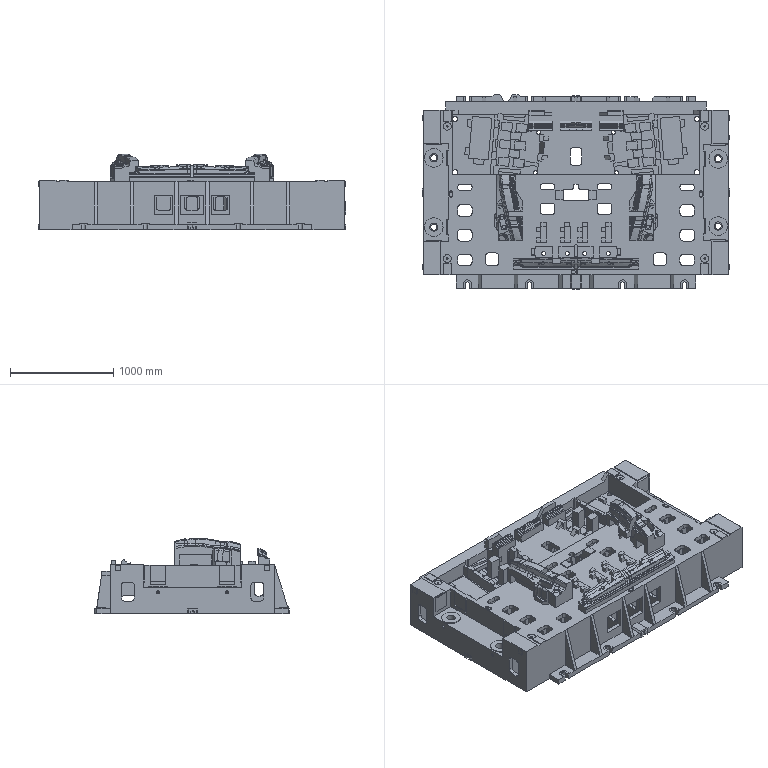Part | NX | features solid 2 | 1 solid | 2897 faces | box 2970 x 1880 x 727.12 mm | volume 739950852 mm3 | plane 1764 | spline 575 | cylinder 558 | commonest cylinder face diameters 60 x457 40 x16 80 x16 30 x14 20 x8 180 x8